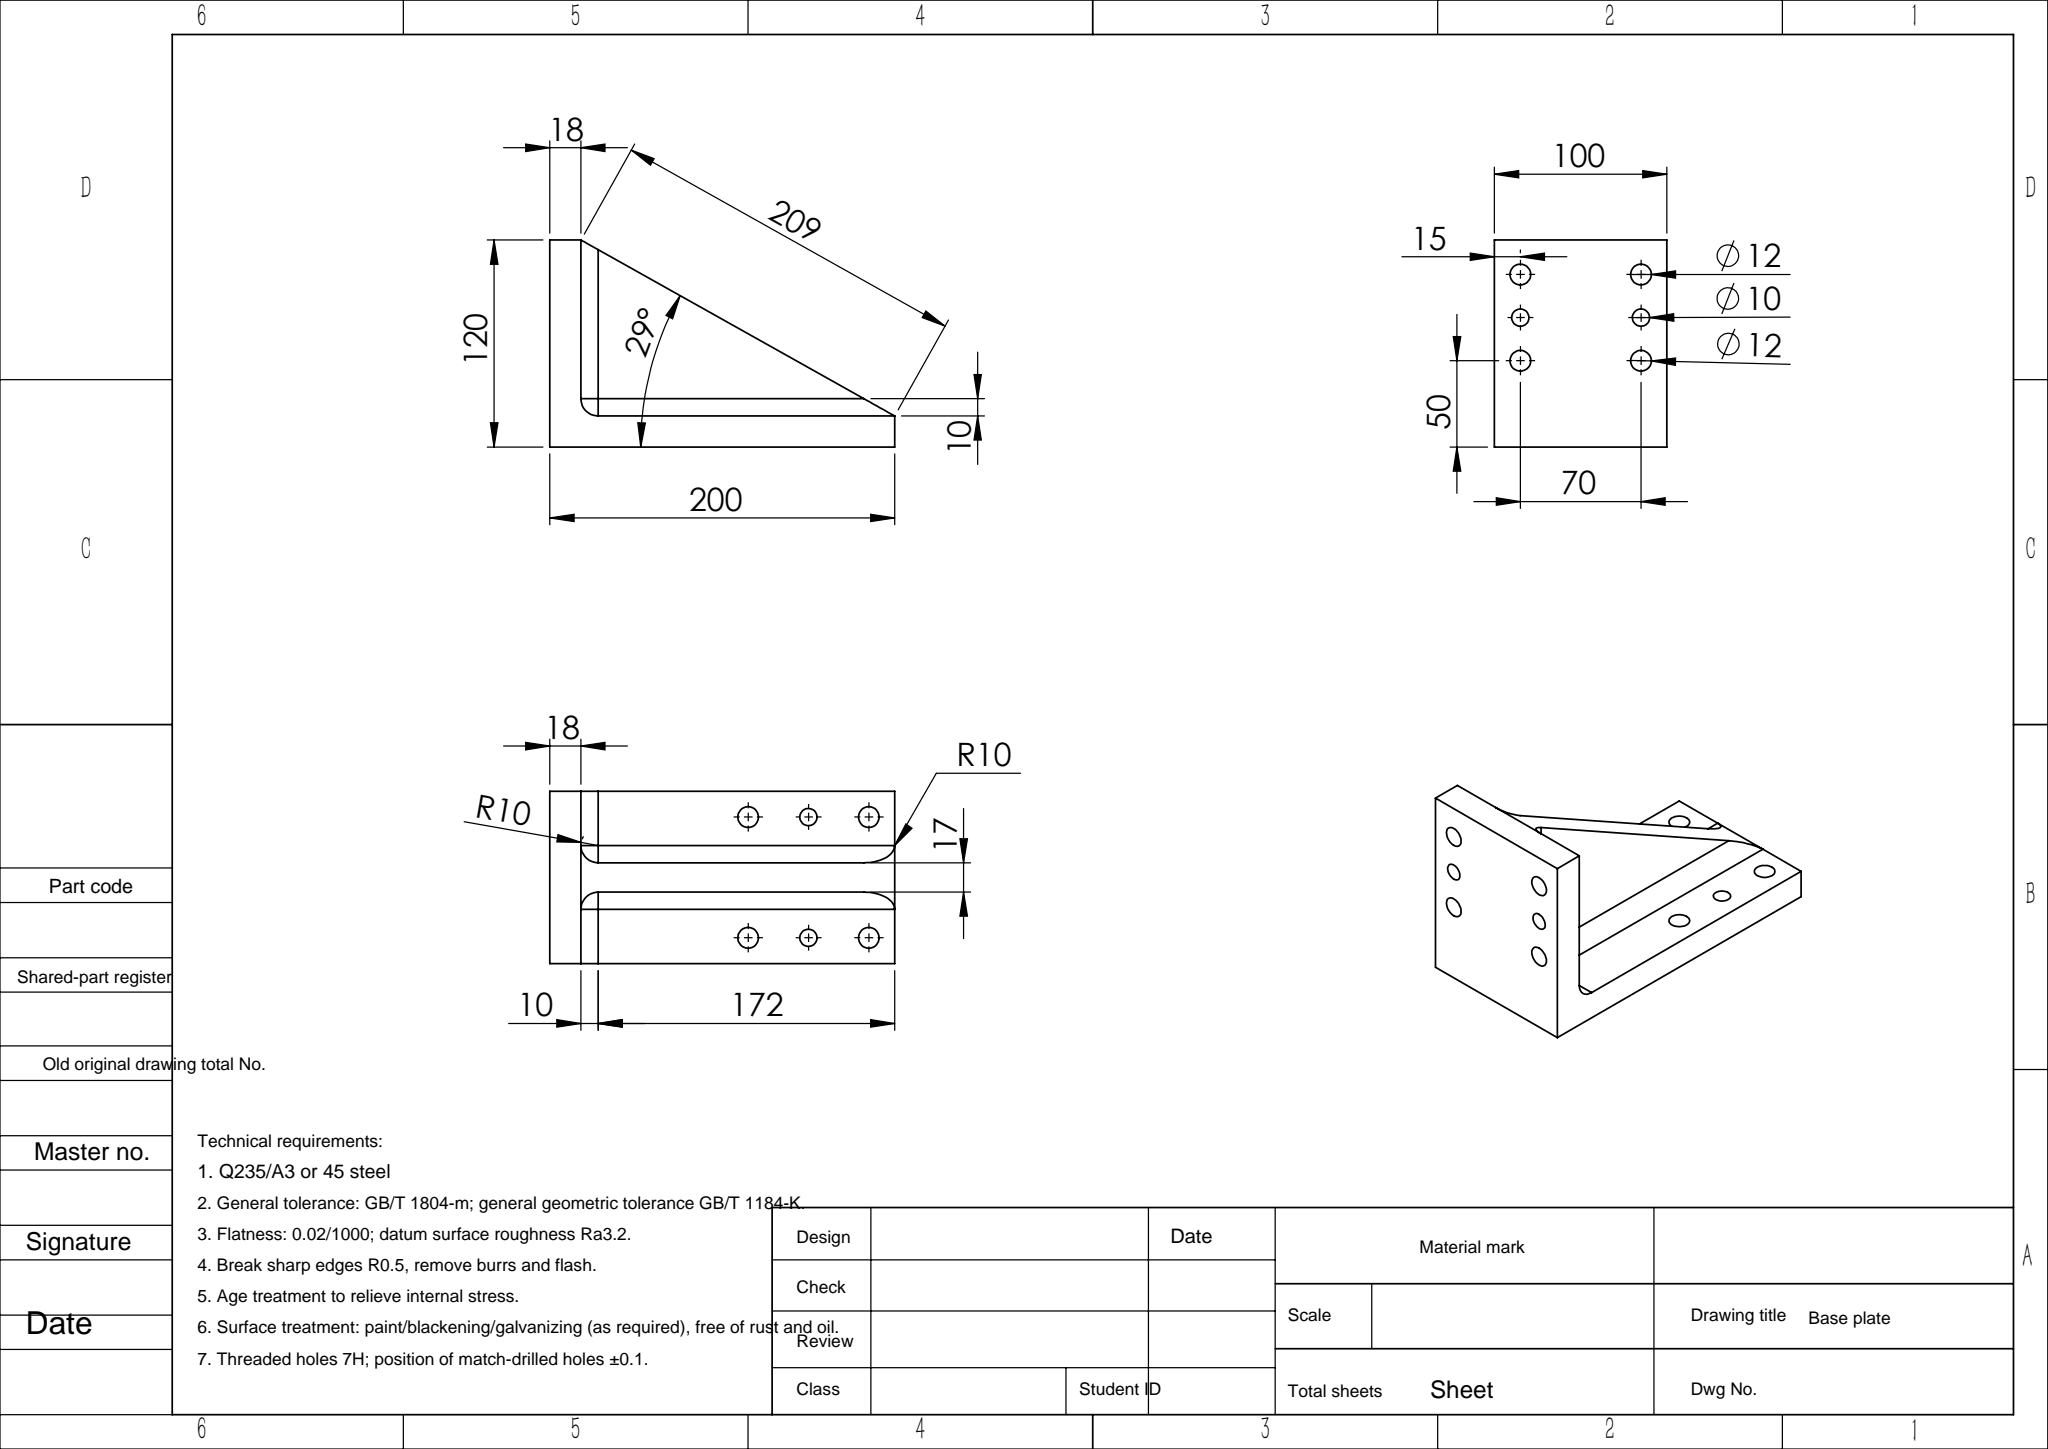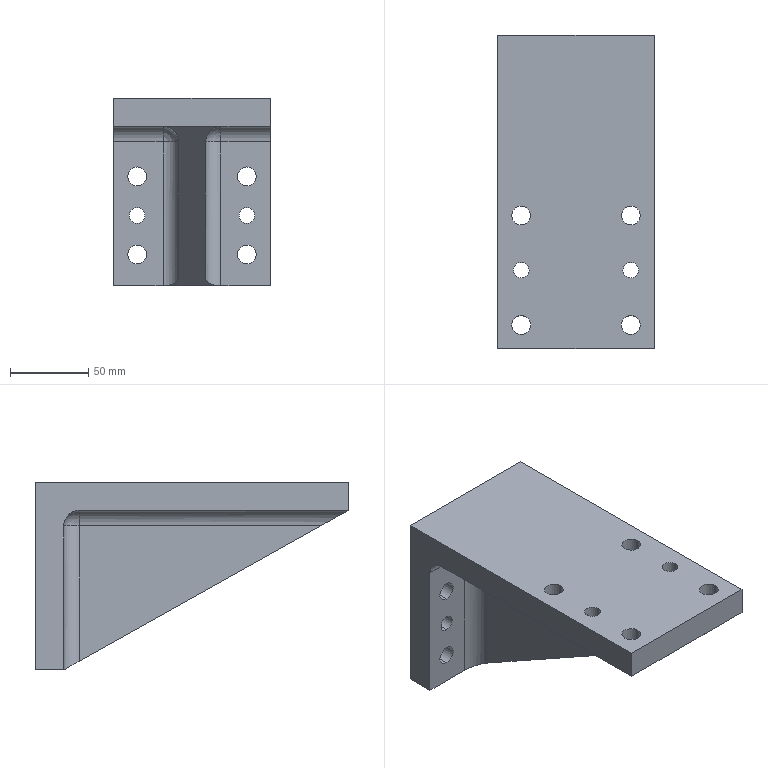Part | SolidWorks | features Fillet 2, ICE 2, Extrusion 1, Rib 1 | 1 solid | 45 faces | box 100 x 200 x 120 mm | volume 692864 mm3 | cylinder 30 | plane 13 | sphere 2 | commonest cylinder face diameters 12 x16 10 x8 20 x6